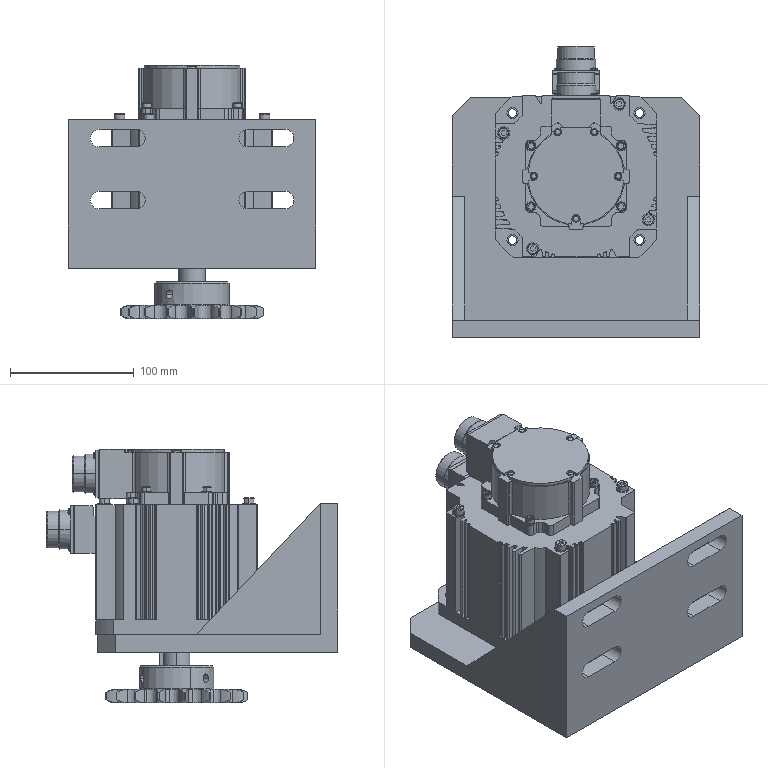Part | SolidWorks | 5 solids | 848 faces | box 200 x 235 x 205 mm | volume 2926314 mm3 | cylinder 413 | plane 303 | spline 82 | cone 50 | commonest cylinder face diameters 1 x90 55.039 x35 2 x30 131 x24 12.191 x23 2.5 x22